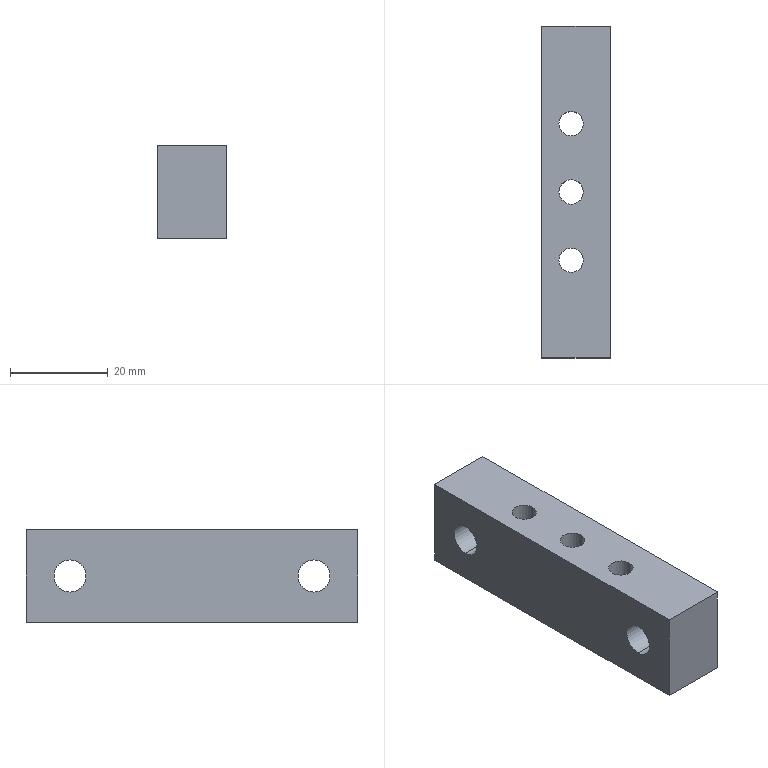Part | STEP file | PN_0047 (fixed plate) | 1 solid | 22 faces | box 14 x 68 x 19 mm | volume 15184 mm3 | cylinder 14 | plane 8 | commonest cylinder face diameters 5 x6 6.6 x4 11 x4